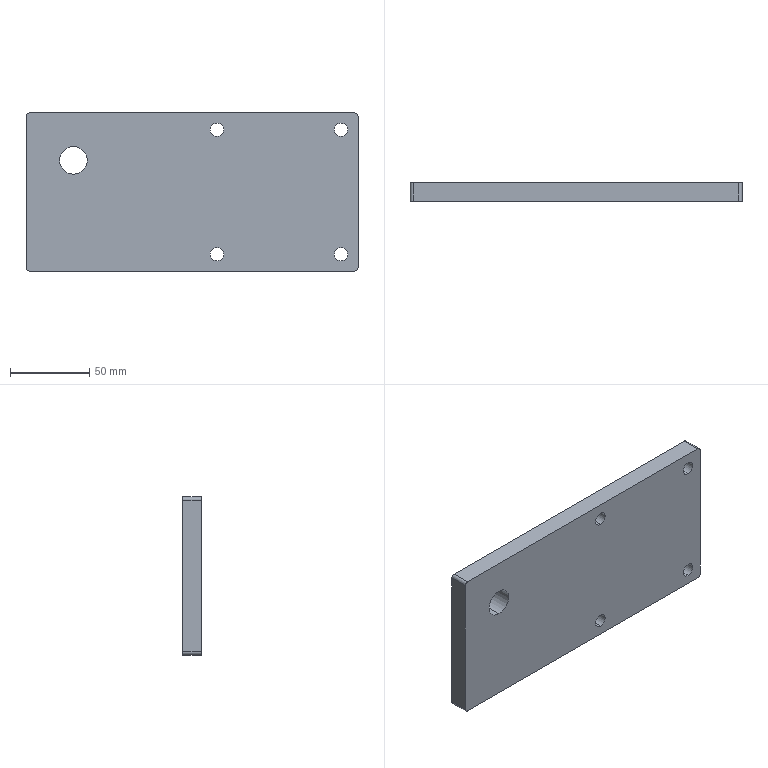Part | SolidWorks | features BaseBody 1 | 1 solid | 20 faces | box 210 x 12 x 100 mm | volume 246349 mm3 | cylinder 14 | plane 6 | commonest cylinder face diameters 8.5 x8 4 x4 17.5 x2
STEP:
#1=CARTESIAN_POINT('',(-75.,0.,11.25));
#2=VERTEX_POINT('',#1);
#3=CARTESIAN_POINT('',(-75.,0.,28.75));
#4=VERTEX_POINT('',#3);
#5=CARTESIAN_POINT('',(-75.,0.,20.));
#6=DIRECTION('',(0.,1.,0.));
#7=DIRECTION('',(0.,0.,1.));
#8=AXIS2_PLACEMENT_3D('',#5,#6,#7);
#9=CIRCLE('',#8,8.75);
#10=EDGE_CURVE('',#2,#4,#9,.T.);
#11=ORIENTED_EDGE('',*,*,#10,.F.);
#12=CARTESIAN_POINT('',(-75.,12.,11.25));
#13=VERTEX_POINT('',#12);
#14=CARTESIAN_POINT('',(-75.,12.,11.25));
#15=DIRECTION('',(0.,1.,0.));
#16=VECTOR('',#15,1000.);
#17=LINE('',#14,#16);
#18=EDGE_CURVE('',#2,#13,#17,.T.);
#19=ORIENTED_EDGE('',*,*,#18,.T.);
#20=CARTESIAN_POINT('',(-75.,12.,28.75));
#21=VERTEX_POINT('',#20);
#22=CARTESIAN_POINT('',(-75.,12.,20.));
#23=DIRECTION('',(0.,-1.,0.));
#24=DIRECTION('',(0.,0.,1.));
#25=AXIS2_PLACEMENT_3D('',#22,#23,#24);
#26=CIRCLE('',#25,8.75);
#27=EDGE_CURVE('',#21,#13,#26,.T.);
#28=ORIENTED_EDGE('',*,*,#27,.F.);
#29=CARTESIAN_POINT('',(-75.,12.,28.75));
#30=DIRECTION('',(0.,1.,0.));
#31=VECTOR('',#30,1000.);
#32=LINE('',#29,#31);
#33=EDGE_CURVE('',#4,#21,#32,.T.);
#34=ORIENTED_EDGE('',*,*,#33,.F.);
#35=EDGE_LOOP('',(#11,#19,#28,#34));
#36=FACE_OUTER_BOUND('',#35,.T.);
#37=CARTESIAN_POINT('',(-75.,12.,20.));
#38=DIRECTION('',(0.,1.,0.));
#39=DIRECTION('',(0.,0.,1.));
#40=AXIS2_PLACEMENT_3D('',#37,#38,#39);
#41=CYLINDRICAL_SURFACE('',#40,8.75);
#42=ADVANCED_FACE('',(#36),#41,.F.);
#43=CARTESIAN_POINT('',(15.75,12.,-35.125));
#44=VERTEX_POINT('',#43);
#45=CARTESIAN_POINT('',(15.75,12.,-43.625));
#46=VERTEX_POINT('',#45);
#47=CARTESIAN_POINT('',(15.75,12.,-39.375));
#48=DIRECTION('',(0.,-1.,0.));
#49=DIRECTION('',(0.,0.,-1.));
#50=AXIS2_PLACEMENT_3D('',#47,#48,#49);
#51=CIRCLE('',#50,4.25);
#52=EDGE_CURVE('',#44,#46,#51,.T.);
#53=ORIENTED_EDGE('',*,*,#52,.F.);
#54=CARTESIAN_POINT('',(15.75,0.,-35.125));
#55=VERTEX_POINT('',#54);
#56=CARTESIAN_POINT('',(15.75,0.,-35.125));
#57=DIRECTION('',(0.,-1.,0.));
#58=VECTOR('',#57,1000.);
#59=LINE('',#56,#58);
#60=EDGE_CURVE('',#44,#55,#59,.T.);
#61=ORIENTED_EDGE('',*,*,#60,.T.);
#62=CARTESIAN_POINT('',(15.75,0.,-43.625));
#63=VERTEX_POINT('',#62);
#64=CARTESIAN_POINT('',(15.75,0.,-39.375));
#65=DIRECTION('',(0.,1.,0.));
#66=DIRECTION('',(0.,0.,-1.));
#67=AXIS2_PLACEMENT_3D('',#64,#65,#66);
#68=CIRCLE('',#67,4.25);
#69=EDGE_CURVE('',#63,#55,#68,.T.);
#70=ORIENTED_EDGE('',*,*,#69,.F.);
#71=CARTESIAN_POINT('',(15.75,0.,-43.625));
#72=DIRECTION('',(0.,-1.,0.));
#73=VECTOR('',#72,1000.);
#74=LINE('',#71,#73);
#75=EDGE_CURVE('',#46,#63,#74,.T.);
#76=ORIENTED_EDGE('',*,*,#75,.F.);
#77=EDGE_LOOP('',(#53,#61,#70,#76));
#78=FACE_OUTER_BOUND('',#77,.T.);
#79=CARTESIAN_POINT('',(15.75,0.,-39.375));
#80=DIRECTION('',(0.,-1.,0.));
#81=DIRECTION('',(0.,0.,-1.));
#82=AXIS2_PLACEMENT_3D('',#79,#80,#81);
#83=CYLINDRICAL_SURFACE('',#82,4.25);
#84=ADVANCED_FACE('',(#78),#83,.F.);
#85=CARTESIAN_POINT('',(94.25,12.,-35.125));
#86=VERTEX_POINT('',#85);
#87=CARTESIAN_POINT('',(94.25,12.,-43.625));
#88=VERTEX_POINT('',#87);
#89=CARTESIAN_POINT('',(94.25,12.,-39.375));
#90=DIRECTION('',(0.,-1.,0.));
#91=DIRECTION('',(0.,0.,-1.));
#92=AXIS2_PLACEMENT_3D('',#89,#90,#91);
#93=CIRCLE('',#92,4.25);
#94=EDGE_CURVE('',#86,#88,#93,.T.);
#95=ORIENTED_EDGE('',*,*,#94,.F.);
#96=CARTESIAN_POINT('',(94.25,0.,-35.125));
#97=VERTEX_POINT('',#96);
#98=CARTESIAN_POINT('',(94.25,0.,-35.125));
#99=DIRECTION('',(0.,-1.,0.));
#100=VECTOR('',#99,1000.);
#101=LINE('',#98,#100);
#102=EDGE_CURVE('',#86,#97,#101,.T.);
#103=ORIENTED_EDGE('',*,*,#102,.T.);
#104=CARTESIAN_POINT('',(94.25,0.,-43.625));
#105=VERTEX_POINT('',#104);
#106=CARTESIAN_POINT('',(94.25,0.,-39.375));
#107=DIRECTION('',(0.,1.,0.));
#108=DIRECTION('',(0.,0.,-1.));
#109=AXIS2_PLACEMENT_3D('',#106,#107,#108);
#110=CIRCLE('',#109,4.25);
#111=EDGE_CURVE('',#105,#97,#110,.T.);
#112=ORIENTED_EDGE('',*,*,#111,.F.);
#113=CARTESIAN_POINT('',(94.25,0.,-43.625));
#114=DIRECTION('',(0.,-1.,0.));
#115=VECTOR('',#114,1000.);
#116=LINE('',#113,#115);
#117=EDGE_CURVE('',#88,#105,#116,.T.);
#118=ORIENTED_EDGE('',*,*,#117,.F.);
#119=EDGE_LOOP('',(#95,#103,#112,#118));
#120=FACE_OUTER_BOUND('',#119,.T.);
#121=CARTESIAN_POINT('',(94.25,0.,-39.375));
#122=DIRECTION('',(0.,-1.,0.));
#123=DIRECTION('',(0.,0.,-1.));
#124=AXIS2_PLACEMENT_3D('',#121,#122,#123);
#125=CYLINDRICAL_SURFACE('',#124,4.25);
#126=ADVANCED_FACE('',(#120),#125,.F.);
#127=CARTESIAN_POINT('',(94.25,12.,43.625));
#128=VERTEX_POINT('',#127);
#129=CARTESIAN_POINT('',(94.25,12.,35.125));
#130=VERTEX_POINT('',#129);
#131=CARTESIAN_POINT('',(94.25,12.,39.375));
#132=DIRECTION('',(0.,-1.,0.));
#133=DIRECTION('',(0.,0.,-1.));
#134=AXIS2_PLACEMENT_3D('',#131,#132,#133);
#135=CIRCLE('',#134,4.25);
#136=EDGE_CURVE('',#128,#130,#135,.T.);
#137=ORIENTED_EDGE('',*,*,#136,.F.);
#138=CARTESIAN_POINT('',(94.25,0.,43.625));
#139=VERTEX_POINT('',#138);
#140=CARTESIAN_POINT('',(94.25,0.,43.625));
#141=DIRECTION('',(0.,-1.,0.));
#142=VECTOR('',#141,1000.);
#143=LINE('',#140,#142);
#144=EDGE_CURVE('',#128,#139,#143,.T.);
#145=ORIENTED_EDGE('',*,*,#144,.T.);
#146=CARTESIAN_POINT('',(94.25,0.,35.125));
#147=VERTEX_POINT('',#146);
#148=CARTESIAN_POINT('',(94.25,0.,39.375));
#149=DIRECTION('',(0.,1.,0.));
#150=DIRECTION('',(0.,0.,-1.));
#151=AXIS2_PLACEMENT_3D('',#148,#149,#150);
#152=CIRCLE('',#151,4.25);
#153=EDGE_CURVE('',#147,#139,#152,.T.);
#154=ORIENTED_EDGE('',*,*,#153,.F.);
#155=CARTESIAN_POINT('',(94.25,0.,35.125));
#156=DIRECTION('',(0.,-1.,0.));
#157=VECTOR('',#156,1000.);
#158=LINE('',#155,#157);
#159=EDGE_CURVE('',#130,#147,#158,.T.);
#160=ORIENTED_EDGE('',*,*,#159,.F.);
#161=EDGE_LOOP('',(#137,#145,#154,#160));
#162=FACE_OUTER_BOUND('',#161,.T.);
#163=CARTESIAN_POINT('',(94.25,0.,39.375));
#164=DIRECTION('',(0.,-1.,0.));
#165=DIRECTION('',(0.,0.,-1.));
#166=AXIS2_PLACEMENT_3D('',#163,#164,#165);
#167=CYLINDRICAL_SURFACE('',#166,4.25);
#168=ADVANCED_FACE('',(#162),#167,.F.);
#169=CARTESIAN_POINT('',(15.75,12.,43.625));
#170=VERTEX_POINT('',#169);
#171=CARTESIAN_POINT('',(15.75,12.,35.125));
#172=VERTEX_POINT('',#171);
#173=CARTESIAN_POINT('',(15.75,12.,39.375));
#174=DIRECTION('',(0.,-1.,0.));
#175=DIRECTION('',(0.,0.,-1.));
#176=AXIS2_PLACEMENT_3D('',#173,#174,#175);
#177=CIRCLE('',#176,4.25);
#178=EDGE_CURVE('',#170,#172,#177,.T.);
#179=ORIENTED_EDGE('',*,*,#178,.F.);
#180=CARTESIAN_POINT('',(15.75,0.,43.625));
#181=VERTEX_POINT('',#180);
#182=CARTESIAN_POINT('',(15.75,0.,43.625));
#183=DIRECTION('',(0.,-1.,0.));
#184=VECTOR('',#183,1000.);
#185=LINE('',#182,#184);
#186=EDGE_CURVE('',#170,#181,#185,.T.);
#187=ORIENTED_EDGE('',*,*,#186,.T.);
#188=CARTESIAN_POINT('',(15.75,0.,35.125));
#189=VERTEX_POINT('',#188);
#190=CARTESIAN_POINT('',(15.75,0.,39.375));
#191=DIRECTION('',(0.,1.,0.));
#192=DIRECTION('',(0.,0.,-1.));
#193=AXIS2_PLACEMENT_3D('',#190,#191,#192);
#194=CIRCLE('',#193,4.25);
#195=EDGE_CURVE('',#189,#181,#194,.T.);
#196=ORIENTED_EDGE('',*,*,#195,.F.);
#197=CARTESIAN_POINT('',(15.75,0.,35.125));
#198=DIRECTION('',(0.,-1.,0.));
#199=VECTOR('',#198,1000.);
#200=LINE('',#197,#199);
#201=EDGE_CURVE('',#172,#189,#200,.T.);
#202=ORIENTED_EDGE('',*,*,#201,.F.);
#203=EDGE_LOOP('',(#179,#187,#196,#202));
#204=FACE_OUTER_BOUND('',#203,.T.);
#205=CARTESIAN_POINT('',(15.75,0.,39.375));
#206=DIRECTION('',(0.,-1.,0.));
#207=DIRECTION('',(0.,0.,-1.));
#208=AXIS2_PLACEMENT_3D('',#205,#206,#207);
#209=CYLINDRICAL_SURFACE('',#208,4.25);
#210=ADVANCED_FACE('',(#204),#209,.F.);
#211=CARTESIAN_POINT('',(103.,0.,50.));
#212=VERTEX_POINT('',#211);
#213=CARTESIAN_POINT('',(-103.,0.,50.));
#214=VERTEX_POINT('',#213);
#215=CARTESIAN_POINT('',(0.,0.,50.));
#216=DIRECTION('',(-1.,0.,0.));
#217=VECTOR('',#216,1000.);
#218=LINE('',#215,#217);
#219=EDGE_CURVE('',#212,#214,#218,.T.);
#220=ORIENTED_EDGE('',*,*,#219,.T.);
#221=CARTESIAN_POINT('',(-105.,0.,48.));
#222=VERTEX_POINT('',#221);
#223=CARTESIAN_POINT('',(-103.,0.,48.));
#224=DIRECTION('',(0.,-1.,0.));
#225=DIRECTION('',(0.,0.,-1.));
#226=AXIS2_PLACEMENT_3D('',#223,#224,#225);
#227=CIRCLE('',#226,2.);
#228=EDGE_CURVE('',#214,#222,#227,.T.);
#229=ORIENTED_EDGE('',*,*,#228,.T.);
#230=CARTESIAN_POINT('',(-105.,0.,-48.));
#231=VERTEX_POINT('',#230);
#232=CARTESIAN_POINT('',(-105.,0.,0.));
#233=DIRECTION('',(0.,0.,-1.));
#234=VECTOR('',#233,1000.);
#235=LINE('',#232,#234);
#236=EDGE_CURVE('',#222,#231,#235,.T.);
#237=ORIENTED_EDGE('',*,*,#236,.T.);
#238=CARTESIAN_POINT('',(-103.,0.,-50.));
#239=VERTEX_POINT('',#238);
#240=CARTESIAN_POINT('',(-103.,0.,-48.));
#241=DIRECTION('',(0.,-1.,0.));
#242=DIRECTION('',(0.,0.,-1.));
#243=AXIS2_PLACEMENT_3D('',#240,#241,#242);
#244=CIRCLE('',#243,2.);
#245=EDGE_CURVE('',#231,#239,#244,.T.);
#246=ORIENTED_EDGE('',*,*,#245,.T.);
#247=CARTESIAN_POINT('',(103.,0.,-50.));
#248=VERTEX_POINT('',#247);
#249=CARTESIAN_POINT('',(0.,0.,-50.));
#250=DIRECTION('',(1.,0.,0.));
#251=VECTOR('',#250,1000.);
#252=LINE('',#249,#251);
#253=EDGE_CURVE('',#239,#248,#252,.T.);
#254=ORIENTED_EDGE('',*,*,#253,.T.);
#255=CARTESIAN_POINT('',(105.,0.,-48.));
#256=VERTEX_POINT('',#255);
#257=CARTESIAN_POINT('',(103.,0.,-48.));
#258=DIRECTION('',(0.,-1.,0.));
#259=DIRECTION('',(0.,0.,-1.));
#260=AXIS2_PLACEMENT_3D('',#257,#258,#259);
#261=CIRCLE('',#260,2.);
#262=EDGE_CURVE('',#248,#256,#261,.T.);
#263=ORIENTED_EDGE('',*,*,#262,.T.);
#264=CARTESIAN_POINT('',(105.,0.,48.));
#265=VERTEX_POINT('',#264);
#266=CARTESIAN_POINT('',(105.,0.,0.));
#267=DIRECTION('',(0.,0.,1.));
#268=VECTOR('',#267,1000.);
#269=LINE('',#266,#268);
#270=EDGE_CURVE('',#256,#265,#269,.T.);
#271=ORIENTED_EDGE('',*,*,#270,.T.);
#272=CARTESIAN_POINT('',(103.,0.,48.));
#273=DIRECTION('',(0.,-1.,0.));
#274=DIRECTION('',(0.,0.,-1.));
#275=AXIS2_PLACEMENT_3D('',#272,#273,#274);
#276=CIRCLE('',#275,2.);
#277=EDGE_CURVE('',#265,#212,#276,.T.);
#278=ORIENTED_EDGE('',*,*,#277,.T.);
#279=EDGE_LOOP('',(#220,#229,#237,#246,#254,#263,#271,#278));
#280=FACE_OUTER_BOUND('',#279,.T.);
#281=CARTESIAN_POINT('',(-75.,0.,20.));
#282=DIRECTION('',(0.,1.,0.));
#283=DIRECTION('',(0.,0.,1.));
#284=AXIS2_PLACEMENT_3D('',#281,#282,#283);
#285=CIRCLE('',#284,8.75);
#286=EDGE_CURVE('',#4,#2,#285,.T.);
#287=ORIENTED_EDGE('',*,*,#286,.T.);
#288=ORIENTED_EDGE('',*,*,#10,.T.);
#289=EDGE_LOOP('',(#287,#288));
#290=FACE_BOUND('',#289,.T.);
#291=ORIENTED_EDGE('',*,*,#69,.T.);
#292=CARTESIAN_POINT('',(15.75,0.,-39.375));
#293=DIRECTION('',(0.,1.,0.));
#294=DIRECTION('',(0.,0.,-1.));
#295=AXIS2_PLACEMENT_3D('',#292,#293,#294);
#296=CIRCLE('',#295,4.25);
#297=EDGE_CURVE('',#55,#63,#296,.T.);
#298=ORIENTED_EDGE('',*,*,#297,.T.);
#299=EDGE_LOOP('',(#291,#298));
#300=FACE_BOUND('',#299,.T.);
#301=ORIENTED_EDGE('',*,*,#111,.T.);
#302=CARTESIAN_POINT('',(94.25,0.,-39.375));
#303=DIRECTION('',(0.,1.,0.));
#304=DIRECTION('',(0.,0.,-1.));
#305=AXIS2_PLACEMENT_3D('',#302,#303,#304);
#306=CIRCLE('',#305,4.25);
#307=EDGE_CURVE('',#97,#105,#306,.T.);
#308=ORIENTED_EDGE('',*,*,#307,.T.);
#309=EDGE_LOOP('',(#301,#308));
#310=FACE_BOUND('',#309,.T.);
#311=ORIENTED_EDGE('',*,*,#153,.T.);
#312=CARTESIAN_POINT('',(94.25,0.,39.375));
#313=DIRECTION('',(0.,1.,0.));
#314=DIRECTION('',(0.,0.,-1.));
#315=AXIS2_PLACEMENT_3D('',#312,#313,#314);
#316=CIRCLE('',#315,4.25);
#317=EDGE_CURVE('',#139,#147,#316,.T.);
#318=ORIENTED_EDGE('',*,*,#317,.T.);
#319=EDGE_LOOP('',(#311,#318));
#320=FACE_BOUND('',#319,.T.);
#321=ORIENTED_EDGE('',*,*,#195,.T.);
#322=CARTESIAN_POINT('',(15.75,0.,39.375));
#323=DIRECTION('',(0.,1.,0.));
#324=DIRECTION('',(0.,0.,-1.));
#325=AXIS2_PLACEMENT_3D('',#322,#323,#324);
#326=CIRCLE('',#325,4.25);
#327=EDGE_CURVE('',#181,#189,#326,.T.);
#328=ORIENTED_EDGE('',*,*,#327,.T.);
#329=EDGE_LOOP('',(#321,#328));
#330=FACE_BOUND('',#329,.T.);
#331=CARTESIAN_POINT('',(0.,0.,0.));
#332=DIRECTION('',(0.,-1.,0.));
#333=DIRECTION('',(0.,0.,-1.));
#334=AXIS2_PLACEMENT_3D('',#331,#332,#333);
#335=PLANE('',#334);
#336=ADVANCED_FACE('',(#280,#290,#300,#310,#320,#330),#335,.T.);
#337=ORIENTED_EDGE('',*,*,#228,.F.);
#338=CARTESIAN_POINT('',(-103.,12.,50.));
#339=VERTEX_POINT('',#338);
#340=CARTESIAN_POINT('',(-103.,12.,50.));
#341=DIRECTION('',(0.,1.,0.));
#342=VECTOR('',#341,1000.);
#343=LINE('',#340,#342);
#344=EDGE_CURVE('',#214,#339,#343,.T.);
#345=ORIENTED_EDGE('',*,*,#344,.T.);
#346=CARTESIAN_POINT('',(-105.,12.,48.));
#347=VERTEX_POINT('',#346);
#348=CARTESIAN_POINT('',(-103.,12.,48.));
#349=DIRECTION('',(0.,-1.,0.));
#350=DIRECTION('',(0.,0.,-1.));
#351=AXIS2_PLACEMENT_3D('',#348,#349,#350);
#352=CIRCLE('',#351,2.);
#353=EDGE_CURVE('',#339,#347,#352,.T.);
#354=ORIENTED_EDGE('',*,*,#353,.T.);
#355=CARTESIAN_POINT('',(-105.,12.,48.));
#356=DIRECTION('',(0.,-1.,0.));
#357=VECTOR('',#356,1000.);
#358=LINE('',#355,#357);
#359=EDGE_CURVE('',#347,#222,#358,.T.);
#360=ORIENTED_EDGE('',*,*,#359,.T.);
#361=EDGE_LOOP('',(#337,#345,#354,#360));
#362=FACE_OUTER_BOUND('',#361,.T.);
#363=CARTESIAN_POINT('',(-103.,12.,48.));
#364=DIRECTION('',(0.,-1.,0.));
#365=DIRECTION('',(0.,0.,-1.));
#366=AXIS2_PLACEMENT_3D('',#363,#364,#365);
#367=CYLINDRICAL_SURFACE('',#366,2.);
#368=ADVANCED_FACE('',(#362),#367,.T.);
#369=CARTESIAN_POINT('',(103.,12.,50.));
#370=VERTEX_POINT('',#369);
#371=CARTESIAN_POINT('',(103.,12.,50.));
#372=DIRECTION('',(0.,-1.,0.));
#373=VECTOR('',#372,1000.);
#374=LINE('',#371,#373);
#375=EDGE_CURVE('',#370,#212,#374,.T.);
#376=ORIENTED_EDGE('',*,*,#375,.F.);
#377=CARTESIAN_POINT('',(-105.,12.,50.));
#378=DIRECTION('',(1.,0.,0.));
#379=VECTOR('',#378,1000.);
#380=LINE('',#377,#379);
#381=EDGE_CURVE('',#339,#370,#380,.T.);
#382=ORIENTED_EDGE('',*,*,#381,.F.);
#383=ORIENTED_EDGE('',*,*,#344,.F.);
#384=ORIENTED_EDGE('',*,*,#219,.F.);
#385=EDGE_LOOP('',(#376,#382,#383,#384));
#386=FACE_OUTER_BOUND('',#385,.T.);
#387=CARTESIAN_POINT('',(-105.,12.,50.));
#388=DIRECTION('',(0.,0.,-1.));
#389=DIRECTION('',(-1.,0.,0.));
#390=AXIS2_PLACEMENT_3D('',#387,#388,#389);
#391=PLANE('',#390);
#392=ADVANCED_FACE('',(#386),#391,.F.);
#393=ORIENTED_EDGE('',*,*,#277,.F.);
#394=CARTESIAN_POINT('',(105.,12.,48.));
#395=VERTEX_POINT('',#394);
#396=CARTESIAN_POINT('',(105.,12.,48.));
#397=DIRECTION('',(0.,1.,0.));
#398=VECTOR('',#397,1000.);
#399=LINE('',#396,#398);
#400=EDGE_CURVE('',#265,#395,#399,.T.);
#401=ORIENTED_EDGE('',*,*,#400,.T.);
#402=CARTESIAN_POINT('',(103.,12.,48.));
#403=DIRECTION('',(0.,-1.,0.));
#404=DIRECTION('',(0.,0.,-1.));
#405=AXIS2_PLACEMENT_3D('',#402,#403,#404);
#406=CIRCLE('',#405,2.);
#407=EDGE_CURVE('',#395,#370,#406,.T.);
#408=ORIENTED_EDGE('',*,*,#407,.T.);
#409=ORIENTED_EDGE('',*,*,#375,.T.);
#410=EDGE_LOOP('',(#393,#401,#408,#409));
#411=FACE_OUTER_BOUND('',#410,.T.);
#412=CARTESIAN_POINT('',(103.,12.,48.));
#413=DIRECTION('',(0.,-1.,0.));
#414=DIRECTION('',(0.,0.,-1.));
#415=AXIS2_PLACEMENT_3D('',#412,#413,#414);
#416=CYLINDRICAL_SURFACE('',#415,2.);
#417=ADVANCED_FACE('',(#411),#416,.T.);
#418=CARTESIAN_POINT('',(105.,12.,-48.));
#419=VERTEX_POINT('',#418);
#420=CARTESIAN_POINT('',(105.,12.,-48.));
#421=DIRECTION('',(0.,-1.,0.));
#422=VECTOR('',#421,1000.);
#423=LINE('',#420,#422);
#424=EDGE_CURVE('',#419,#256,#423,.T.);
#425=ORIENTED_EDGE('',*,*,#424,.F.);
#426=CARTESIAN_POINT('',(105.,12.,50.));
#427=DIRECTION('',(0.,0.,-1.));
#428=VECTOR('',#427,1000.);
#429=LINE('',#426,#428);
#430=EDGE_CURVE('',#395,#419,#429,.T.);
#431=ORIENTED_EDGE('',*,*,#430,.F.);
#432=ORIENTED_EDGE('',*,*,#400,.F.);
#433=ORIENTED_EDGE('',*,*,#270,.F.);
#434=EDGE_LOOP('',(#425,#431,#432,#433));
#435=FACE_OUTER_BOUND('',#434,.T.);
#436=CARTESIAN_POINT('',(105.,12.,50.));
#437=DIRECTION('',(-1.,0.,0.));
#438=DIRECTION('',(0.,0.,1.));
#439=AXIS2_PLACEMENT_3D('',#436,#437,#438);
#440=PLANE('',#439);
#441=ADVANCED_FACE('',(#435),#440,.F.);
#442=ORIENTED_EDGE('',*,*,#262,.F.);
#443=CARTESIAN_POINT('',(103.,12.,-50.));
#444=VERTEX_POINT('',#443);
#445=CARTESIAN_POINT('',(103.,12.,-50.));
#446=DIRECTION('',(0.,1.,0.));
#447=VECTOR('',#446,1000.);
#448=LINE('',#445,#447);
#449=EDGE_CURVE('',#248,#444,#448,.T.);
#450=ORIENTED_EDGE('',*,*,#449,.T.);
#451=CARTESIAN_POINT('',(103.,12.,-48.));
#452=DIRECTION('',(0.,-1.,0.));
#453=DIRECTION('',(0.,0.,-1.));
#454=AXIS2_PLACEMENT_3D('',#451,#452,#453);
#455=CIRCLE('',#454,2.);
#456=EDGE_CURVE('',#444,#419,#455,.T.);
#457=ORIENTED_EDGE('',*,*,#456,.T.);
#458=ORIENTED_EDGE('',*,*,#424,.T.);
#459=EDGE_LOOP('',(#442,#450,#457,#458));
#460=FACE_OUTER_BOUND('',#459,.T.);
#461=CARTESIAN_POINT('',(103.,12.,-48.));
#462=DIRECTION('',(0.,-1.,0.));
#463=DIRECTION('',(0.,0.,-1.));
#464=AXIS2_PLACEMENT_3D('',#461,#462,#463);
#465=CYLINDRICAL_SURFACE('',#464,2.);
#466=ADVANCED_FACE('',(#460),#465,.T.);
#467=CARTESIAN_POINT('',(-103.,12.,-50.));
#468=VERTEX_POINT('',#467);
#469=CARTESIAN_POINT('',(-103.,12.,-50.));
#470=DIRECTION('',(0.,-1.,0.));
#471=VECTOR('',#470,1000.);
#472=LINE('',#469,#471);
#473=EDGE_CURVE('',#468,#239,#472,.T.);
#474=ORIENTED_EDGE('',*,*,#473,.F.);
#475=CARTESIAN_POINT('',(-105.,12.,-50.));
#476=DIRECTION('',(-1.,0.,0.));
#477=VECTOR('',#476,1000.);
#478=LINE('',#475,#477);
#479=EDGE_CURVE('',#444,#468,#478,.T.);
#480=ORIENTED_EDGE('',*,*,#479,.F.);
#481=ORIENTED_EDGE('',*,*,#449,.F.);
#482=ORIENTED_EDGE('',*,*,#253,.F.);
#483=EDGE_LOOP('',(#474,#480,#481,#482));
#484=FACE_OUTER_BOUND('',#483,.T.);
#485=CARTESIAN_POINT('',(-105.,12.,-50.));
#486=DIRECTION('',(0.,0.,1.));
#487=DIRECTION('',(1.,0.,0.));
#488=AXIS2_PLACEMENT_3D('',#485,#486,#487);
#489=PLANE('',#488);
#490=ADVANCED_FACE('',(#484),#489,.F.);
#491=ORIENTED_EDGE('',*,*,#245,.F.);
#492=CARTESIAN_POINT('',(-105.,12.,-48.));
#493=VERTEX_POINT('',#492);
#494=CARTESIAN_POINT('',(-105.,12.,-48.));
#495=DIRECTION('',(0.,1.,0.));
#496=VECTOR('',#495,1000.);
#497=LINE('',#494,#496);
#498=EDGE_CURVE('',#231,#493,#497,.T.);
#499=ORIENTED_EDGE('',*,*,#498,.T.);
#500=CARTESIAN_POINT('',(-103.,12.,-48.));
#501=DIRECTION('',(0.,-1.,0.));
#502=DIRECTION('',(0.,0.,-1.));
#503=AXIS2_PLACEMENT_3D('',#500,#501,#502);
#504=CIRCLE('',#503,2.);
#505=EDGE_CURVE('',#493,#468,#504,.T.);
#506=ORIENTED_EDGE('',*,*,#505,.T.);
#507=ORIENTED_EDGE('',*,*,#473,.T.);
#508=EDGE_LOOP('',(#491,#499,#506,#507));
#509=FACE_OUTER_BOUND('',#508,.T.);
#510=CARTESIAN_POINT('',(-103.,12.,-48.));
#511=DIRECTION('',(0.,-1.,0.));
#512=DIRECTION('',(0.,0.,-1.));
#513=AXIS2_PLACEMENT_3D('',#510,#511,#512);
#514=CYLINDRICAL_SURFACE('',#513,2.);
#515=ADVANCED_FACE('',(#509),#514,.T.);
#516=ORIENTED_EDGE('',*,*,#498,.F.);
#517=ORIENTED_EDGE('',*,*,#236,.F.);
#518=ORIENTED_EDGE('',*,*,#359,.F.);
#519=CARTESIAN_POINT('',(-105.,12.,50.));
#520=DIRECTION('',(0.,0.,1.));
#521=VECTOR('',#520,1000.);
#522=LINE('',#519,#521);
#523=EDGE_CURVE('',#493,#347,#522,.T.);
#524=ORIENTED_EDGE('',*,*,#523,.F.);
#525=EDGE_LOOP('',(#516,#517,#518,#524));
#526=FACE_OUTER_BOUND('',#525,.T.);
#527=CARTESIAN_POINT('',(-105.,12.,50.));
#528=DIRECTION('',(1.,0.,0.));
#529=DIRECTION('',(0.,0.,-1.));
#530=AXIS2_PLACEMENT_3D('',#527,#528,#529);
#531=PLANE('',#530);
#532=ADVANCED_FACE('',(#526),#531,.F.);
#533=ORIENTED_EDGE('',*,*,#18,.F.);
#534=ORIENTED_EDGE('',*,*,#286,.F.);
#535=ORIENTED_EDGE('',*,*,#33,.T.);
#536=CARTESIAN_POINT('',(-75.,12.,20.));
#537=DIRECTION('',(0.,-1.,0.));
#538=DIRECTION('',(0.,0.,1.));
#539=AXIS2_PLACEMENT_3D('',#536,#537,#538);
#540=CIRCLE('',#539,8.75);
#541=EDGE_CURVE('',#13,#21,#540,.T.);
#542=ORIENTED_EDGE('',*,*,#541,.F.);
#543=EDGE_LOOP('',(#533,#534,#535,#542));
#544=FACE_OUTER_BOUND('',#543,.T.);
#545=CARTESIAN_POINT('',(-75.,12.,20.));
#546=DIRECTION('',(0.,1.,0.));
#547=DIRECTION('',(0.,0.,1.));
#548=AXIS2_PLACEMENT_3D('',#545,#546,#547);
#549=CYLINDRICAL_SURFACE('',#548,8.75);
#550=ADVANCED_FACE('',(#544),#549,.F.);
#551=ORIENTED_EDGE('',*,*,#60,.F.);
#552=CARTESIAN_POINT('',(15.75,12.,-39.375));
#553=DIRECTION('',(0.,-1.,0.));
#554=DIRECTION('',(0.,0.,-1.));
#555=AXIS2_PLACEMENT_3D('',#552,#553,#554);
#556=CIRCLE('',#555,4.25);
#557=EDGE_CURVE('',#46,#44,#556,.T.);
#558=ORIENTED_EDGE('',*,*,#557,.F.);
#559=ORIENTED_EDGE('',*,*,#75,.T.);
#560=ORIENTED_EDGE('',*,*,#297,.F.);
#561=EDGE_LOOP('',(#551,#558,#559,#560));
#562=FACE_OUTER_BOUND('',#561,.T.);
#563=CARTESIAN_POINT('',(15.75,0.,-39.375));
#564=DIRECTION('',(0.,-1.,0.));
#565=DIRECTION('',(0.,0.,-1.));
#566=AXIS2_PLACEMENT_3D('',#563,#564,#565);
#567=CYLINDRICAL_SURFACE('',#566,4.25);
#568=ADVANCED_FACE('',(#562),#567,.F.);
#569=ORIENTED_EDGE('',*,*,#102,.F.);
#570=CARTESIAN_POINT('',(94.25,12.,-39.375));
#571=DIRECTION('',(0.,-1.,0.));
#572=DIRECTION('',(0.,0.,-1.));
#573=AXIS2_PLACEMENT_3D('',#570,#571,#572);
#574=CIRCLE('',#573,4.25);
#575=EDGE_CURVE('',#88,#86,#574,.T.);
#576=ORIENTED_EDGE('',*,*,#575,.F.);
#577=ORIENTED_EDGE('',*,*,#117,.T.);
#578=ORIENTED_EDGE('',*,*,#307,.F.);
#579=EDGE_LOOP('',(#569,#576,#577,#578));
#580=FACE_OUTER_BOUND('',#579,.T.);
#581=CARTESIAN_POINT('',(94.25,0.,-39.375));
#582=DIRECTION('',(0.,-1.,0.));
#583=DIRECTION('',(0.,0.,-1.));
#584=AXIS2_PLACEMENT_3D('',#581,#582,#583);
#585=CYLINDRICAL_SURFACE('',#584,4.25);
#586=ADVANCED_FACE('',(#580),#585,.F.);
#587=ORIENTED_EDGE('',*,*,#144,.F.);
#588=CARTESIAN_POINT('',(94.25,12.,39.375));
#589=DIRECTION('',(0.,-1.,0.));
#590=DIRECTION('',(0.,0.,-1.));
#591=AXIS2_PLACEMENT_3D('',#588,#589,#590);
#592=CIRCLE('',#591,4.25);
#593=EDGE_CURVE('',#130,#128,#592,.T.);
#594=ORIENTED_EDGE('',*,*,#593,.F.);
#595=ORIENTED_EDGE('',*,*,#159,.T.);
#596=ORIENTED_EDGE('',*,*,#317,.F.);
#597=EDGE_LOOP('',(#587,#594,#595,#596));
#598=FACE_OUTER_BOUND('',#597,.T.);
#599=CARTESIAN_POINT('',(94.25,0.,39.375));
#600=DIRECTION('',(0.,-1.,0.));
#601=DIRECTION('',(0.,0.,-1.));
#602=AXIS2_PLACEMENT_3D('',#599,#600,#601);
#603=CYLINDRICAL_SURFACE('',#602,4.25);
#604=ADVANCED_FACE('',(#598),#603,.F.);
#605=ORIENTED_EDGE('',*,*,#186,.F.);
#606=CARTESIAN_POINT('',(15.75,12.,39.375));
#607=DIRECTION('',(0.,-1.,0.));
#608=DIRECTION('',(0.,0.,-1.));
#609=AXIS2_PLACEMENT_3D('',#606,#607,#608);
#610=CIRCLE('',#609,4.25);
#611=EDGE_CURVE('',#172,#170,#610,.T.);
#612=ORIENTED_EDGE('',*,*,#611,.F.);
#613=ORIENTED_EDGE('',*,*,#201,.T.);
#614=ORIENTED_EDGE('',*,*,#327,.F.);
#615=EDGE_LOOP('',(#605,#612,#613,#614));
#616=FACE_OUTER_BOUND('',#615,.T.);
#617=CARTESIAN_POINT('',(15.75,0.,39.375));
#618=DIRECTION('',(0.,-1.,0.));
#619=DIRECTION('',(0.,0.,-1.));
#620=AXIS2_PLACEMENT_3D('',#617,#618,#619);
#621=CYLINDRICAL_SURFACE('',#620,4.25);
#622=ADVANCED_FACE('',(#616),#621,.F.);
#623=ORIENTED_EDGE('',*,*,#505,.F.);
#624=ORIENTED_EDGE('',*,*,#523,.T.);
#625=ORIENTED_EDGE('',*,*,#353,.F.);
#626=ORIENTED_EDGE('',*,*,#381,.T.);
#627=ORIENTED_EDGE('',*,*,#407,.F.);
#628=ORIENTED_EDGE('',*,*,#430,.T.);
#629=ORIENTED_EDGE('',*,*,#456,.F.);
#630=ORIENTED_EDGE('',*,*,#479,.T.);
#631=EDGE_LOOP('',(#623,#624,#625,#626,#627,#628,#629,#630));
#632=FACE_OUTER_BOUND('',#631,.T.);
#633=ORIENTED_EDGE('',*,*,#27,.T.);
#634=ORIENTED_EDGE('',*,*,#541,.T.);
#635=EDGE_LOOP('',(#633,#634));
#636=FACE_BOUND('',#635,.T.);
#637=ORIENTED_EDGE('',*,*,#557,.T.);
#638=ORIENTED_EDGE('',*,*,#52,.T.);
#639=EDGE_LOOP('',(#637,#638));
#640=FACE_BOUND('',#639,.T.);
#641=ORIENTED_EDGE('',*,*,#575,.T.);
#642=ORIENTED_EDGE('',*,*,#94,.T.);
#643=EDGE_LOOP('',(#641,#642));
#644=FACE_BOUND('',#643,.T.);
#645=ORIENTED_EDGE('',*,*,#593,.T.);
#646=ORIENTED_EDGE('',*,*,#136,.T.);
#647=EDGE_LOOP('',(#645,#646));
#648=FACE_BOUND('',#647,.T.);
#649=ORIENTED_EDGE('',*,*,#611,.T.);
#650=ORIENTED_EDGE('',*,*,#178,.T.);
#651=EDGE_LOOP('',(#649,#650));
#652=FACE_BOUND('',#651,.T.);
#653=CARTESIAN_POINT('',(0.,12.,0.));
#654=DIRECTION('',(0.,-1.,0.));
#655=DIRECTION('',(0.,0.,-1.));
#656=AXIS2_PLACEMENT_3D('',#653,#654,#655);
#657=PLANE('',#656);
#658=ADVANCED_FACE('',(#632,#636,#640,#644,#648,#652),#657,.F.);
#659=CLOSED_SHELL('',(#42,#84,#126,#168,#210,#336,#368,#392,#417,#441,#466,#490,#515,#532,#550,#568,#586,#604,#622,#658));
#660=MANIFOLD_SOLID_BREP('',#659);
#661=CARTESIAN_POINT('',(0.,0.,0.));
#662=DIRECTION('',(0.,0.,1.));
#663=DIRECTION('',(1.,0.,0.));
#664=AXIS2_PLACEMENT_3D('',#661,#662,#663);
#665=(LENGTH_UNIT()NAMED_UNIT(*)SI_UNIT(.MILLI.,.METRE.));
#666=UNCERTAINTY_MEASURE_WITH_UNIT(LENGTH_MEASURE(0.00001),#665,'','');
#667=(NAMED_UNIT(*)PLANE_ANGLE_UNIT()SI_UNIT($,.RADIAN.));
#668=(NAMED_UNIT(*)SI_UNIT($,.STERADIAN.)SOLID_ANGLE_UNIT());
#669=(GEOMETRIC_REPRESENTATION_CONTEXT(3)GLOBAL_UNCERTAINTY_ASSIGNED_CONTEXT((#666))GLOBAL_UNIT_ASSIGNED_CONTEXT((#665,#667,#668))REPRESENTATION_CONTEXT('',''));
#670=ADVANCED_BREP_SHAPE_REPRESENTATION('',(#660,#664),#669);